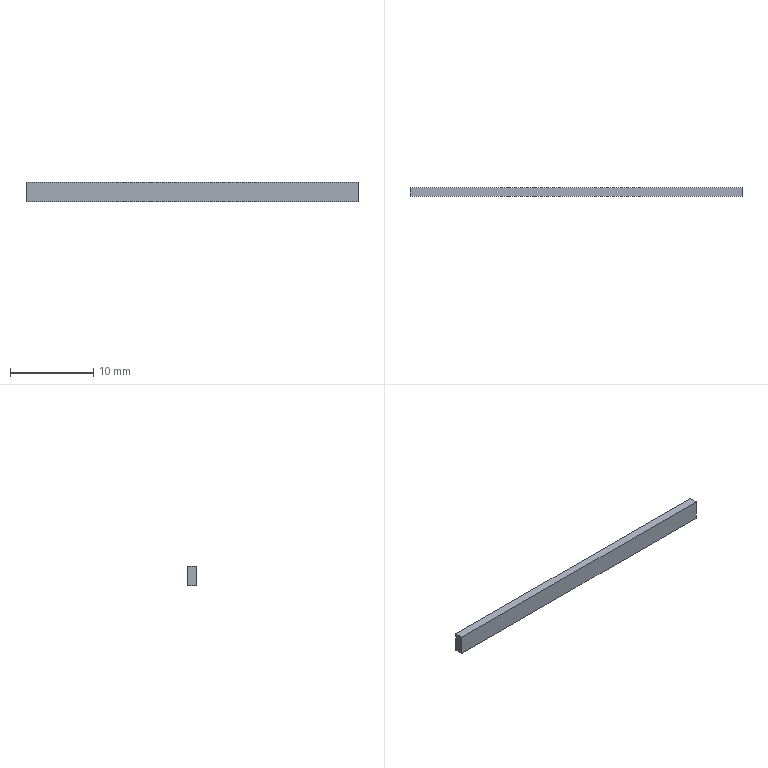Part | STEP file | TKR26H40-STAS | 1 solid | 6 faces | box 40 x 1 x 2.4 mm | volume 96 mm3 | plane 6
STEP:
#1=CARTESIAN_POINT('',(0.,0.,0.));
#2=DIRECTION('',(0.,0.,1.));
#3=DIRECTION('',(1.,0.,0.));
#4=AXIS2_PLACEMENT_3D('',#1,#2,#3);
#5=CARTESIAN_POINT('',(0.,40.,0.));
#6=VERTEX_POINT('',#5);
#7=CARTESIAN_POINT('',(0.,39.,0.));
#8=VERTEX_POINT('',#7);
#9=CARTESIAN_POINT('',(0.,39.5,0.));
#10=DIRECTION('',(0.,-1.,0.));
#11=VECTOR('',#10,1.);
#12=LINE('',#9,#11);
#13=CARTESIAN_POINT('',(20.,39.5,0.));
#14=DIRECTION('',(0.,0.,-1.));
#15=DIRECTION('',(0.,1.,0.));
#16=AXIS2_PLACEMENT_3D('',#13,#14,#15);
#17=PLANE('',#16);
#18=CARTESIAN_POINT('',(0.,-20.));
#19=DIRECTION('',(-1.,0.));
#20=VECTOR('',#19,1.);
#21=LINE('',#18,#20);
#22=(GEOMETRIC_REPRESENTATION_CONTEXT(2)PARAMETRIC_REPRESENTATION_CONTEXT()REPRESENTATION_CONTEXT('',''));
#23=DEFINITIONAL_REPRESENTATION('',(#21),#22);
#24=PCURVE('',#17,#23);
#25=CARTESIAN_POINT('',(0.,39.5,2.4));
#26=DIRECTION('',(-1.,0.,0.));
#27=DIRECTION('',(0.,0.,1.));
#28=AXIS2_PLACEMENT_3D('',#25,#26,#27);
#29=PLANE('',#28);
#30=CARTESIAN_POINT('',(-2.4,0.));
#31=DIRECTION('',(0.,-1.));
#32=VECTOR('',#31,1.);
#33=LINE('',#30,#32);
#34=(GEOMETRIC_REPRESENTATION_CONTEXT(2)PARAMETRIC_REPRESENTATION_CONTEXT()REPRESENTATION_CONTEXT('',''));
#35=DEFINITIONAL_REPRESENTATION('',(#33),#34);
#36=PCURVE('',#29,#35);
#37=SURFACE_CURVE('',#12,(#24,#36),.PCURVE_S1.);
#38=EDGE_CURVE('',#6,#8,#37,.T.);
#39=ORIENTED_EDGE('',*,*,#38,.F.);
#40=CARTESIAN_POINT('',(40.,40.,0.));
#41=VERTEX_POINT('',#40);
#42=CARTESIAN_POINT('',(20.,40.,0.));
#43=DIRECTION('',(-1.,0.,0.));
#44=VECTOR('',#43,1.);
#45=LINE('',#42,#44);
#46=CARTESIAN_POINT('',(0.5,0.));
#47=DIRECTION('',(0.,-1.));
#48=VECTOR('',#47,1.);
#49=LINE('',#46,#48);
#50=(GEOMETRIC_REPRESENTATION_CONTEXT(2)PARAMETRIC_REPRESENTATION_CONTEXT()REPRESENTATION_CONTEXT('',''));
#51=DEFINITIONAL_REPRESENTATION('',(#49),#50);
#52=PCURVE('',#17,#51);
#53=CARTESIAN_POINT('',(20.,40.,2.4));
#54=DIRECTION('',(0.,1.,0.));
#55=DIRECTION('',(0.,0.,1.));
#56=AXIS2_PLACEMENT_3D('',#53,#54,#55);
#57=PLANE('',#56);
#58=CARTESIAN_POINT('',(-2.4,0.));
#59=DIRECTION('',(0.,-1.));
#60=VECTOR('',#59,1.);
#61=LINE('',#58,#60);
#62=(GEOMETRIC_REPRESENTATION_CONTEXT(2)PARAMETRIC_REPRESENTATION_CONTEXT()REPRESENTATION_CONTEXT('',''));
#63=DEFINITIONAL_REPRESENTATION('',(#61),#62);
#64=PCURVE('',#57,#63);
#65=SURFACE_CURVE('',#45,(#52,#64),.PCURVE_S1.);
#66=EDGE_CURVE('',#41,#6,#65,.T.);
#67=ORIENTED_EDGE('',*,*,#66,.F.);
#68=CARTESIAN_POINT('',(40.,39.,0.));
#69=VERTEX_POINT('',#68);
#70=CARTESIAN_POINT('',(40.,39.5,0.));
#71=DIRECTION('',(0.,1.,0.));
#72=VECTOR('',#71,1.);
#73=LINE('',#70,#72);
#74=CARTESIAN_POINT('',(0.,20.));
#75=DIRECTION('',(1.,0.));
#76=VECTOR('',#75,1.);
#77=LINE('',#74,#76);
#78=(GEOMETRIC_REPRESENTATION_CONTEXT(2)PARAMETRIC_REPRESENTATION_CONTEXT()REPRESENTATION_CONTEXT('',''));
#79=DEFINITIONAL_REPRESENTATION('',(#77),#78);
#80=PCURVE('',#17,#79);
#81=CARTESIAN_POINT('',(40.,39.5,2.4));
#82=DIRECTION('',(1.,0.,0.));
#83=DIRECTION('',(0.,0.,-1.));
#84=AXIS2_PLACEMENT_3D('',#81,#82,#83);
#85=PLANE('',#84);
#86=CARTESIAN_POINT('',(2.4,0.));
#87=DIRECTION('',(0.,1.));
#88=VECTOR('',#87,1.);
#89=LINE('',#86,#88);
#90=(GEOMETRIC_REPRESENTATION_CONTEXT(2)PARAMETRIC_REPRESENTATION_CONTEXT()REPRESENTATION_CONTEXT('',''));
#91=DEFINITIONAL_REPRESENTATION('',(#89),#90);
#92=PCURVE('',#85,#91);
#93=SURFACE_CURVE('',#73,(#80,#92),.PCURVE_S1.);
#94=EDGE_CURVE('',#69,#41,#93,.T.);
#95=ORIENTED_EDGE('',*,*,#94,.F.);
#96=CARTESIAN_POINT('',(20.,39.,0.));
#97=DIRECTION('',(1.,0.,0.));
#98=VECTOR('',#97,1.);
#99=LINE('',#96,#98);
#100=CARTESIAN_POINT('',(-0.5,0.));
#101=DIRECTION('',(0.,1.));
#102=VECTOR('',#101,1.);
#103=LINE('',#100,#102);
#104=(GEOMETRIC_REPRESENTATION_CONTEXT(2)PARAMETRIC_REPRESENTATION_CONTEXT()REPRESENTATION_CONTEXT('',''));
#105=DEFINITIONAL_REPRESENTATION('',(#103),#104);
#106=PCURVE('',#17,#105);
#107=CARTESIAN_POINT('',(20.,39.,2.4));
#108=DIRECTION('',(0.,-1.,0.));
#109=DIRECTION('',(0.,0.,-1.));
#110=AXIS2_PLACEMENT_3D('',#107,#108,#109);
#111=PLANE('',#110);
#112=CARTESIAN_POINT('',(2.4,0.));
#113=DIRECTION('',(0.,1.));
#114=VECTOR('',#113,1.);
#115=LINE('',#112,#114);
#116=(GEOMETRIC_REPRESENTATION_CONTEXT(2)PARAMETRIC_REPRESENTATION_CONTEXT()REPRESENTATION_CONTEXT('',''));
#117=DEFINITIONAL_REPRESENTATION('',(#115),#116);
#118=PCURVE('',#111,#117);
#119=SURFACE_CURVE('',#99,(#106,#118),.PCURVE_S1.);
#120=EDGE_CURVE('',#8,#69,#119,.T.);
#121=ORIENTED_EDGE('',*,*,#120,.F.);
#122=EDGE_LOOP('',(#39,#67,#95,#121));
#123=FACE_BOUND('',#122,.T.);
#124=ADVANCED_FACE('',(#123),#17,.T.);
#125=CARTESIAN_POINT('',(0.,40.,2.4));
#126=VERTEX_POINT('',#125);
#127=CARTESIAN_POINT('',(0.,40.,2.4));
#128=DIRECTION('',(0.,0.,-1.));
#129=VECTOR('',#128,1.);
#130=LINE('',#127,#129);
#131=CARTESIAN_POINT('',(0.,0.5));
#132=DIRECTION('',(-1.,0.));
#133=VECTOR('',#132,1.);
#134=LINE('',#131,#133);
#135=(GEOMETRIC_REPRESENTATION_CONTEXT(2)PARAMETRIC_REPRESENTATION_CONTEXT()REPRESENTATION_CONTEXT('',''));
#136=DEFINITIONAL_REPRESENTATION('',(#134),#135);
#137=PCURVE('',#29,#136);
#138=CARTESIAN_POINT('',(0.,-20.));
#139=DIRECTION('',(-1.,0.));
#140=VECTOR('',#139,1.);
#141=LINE('',#138,#140);
#142=(GEOMETRIC_REPRESENTATION_CONTEXT(2)PARAMETRIC_REPRESENTATION_CONTEXT()REPRESENTATION_CONTEXT('',''));
#143=DEFINITIONAL_REPRESENTATION('',(#141),#142);
#144=PCURVE('',#57,#143);
#145=SURFACE_CURVE('',#130,(#137,#144),.PCURVE_S1.);
#146=EDGE_CURVE('',#126,#6,#145,.T.);
#147=ORIENTED_EDGE('',*,*,#146,.T.);
#148=ORIENTED_EDGE('',*,*,#38,.T.);
#149=CARTESIAN_POINT('',(0.,39.,2.4));
#150=VERTEX_POINT('',#149);
#151=CARTESIAN_POINT('',(0.,39.,2.4));
#152=DIRECTION('',(0.,0.,-1.));
#153=VECTOR('',#152,1.);
#154=LINE('',#151,#153);
#155=CARTESIAN_POINT('',(0.,-0.5));
#156=DIRECTION('',(-1.,0.));
#157=VECTOR('',#156,1.);
#158=LINE('',#155,#157);
#159=(GEOMETRIC_REPRESENTATION_CONTEXT(2)PARAMETRIC_REPRESENTATION_CONTEXT()REPRESENTATION_CONTEXT('',''));
#160=DEFINITIONAL_REPRESENTATION('',(#158),#159);
#161=PCURVE('',#29,#160);
#162=CARTESIAN_POINT('',(0.,-20.));
#163=DIRECTION('',(1.,0.));
#164=VECTOR('',#163,1.);
#165=LINE('',#162,#164);
#166=(GEOMETRIC_REPRESENTATION_CONTEXT(2)PARAMETRIC_REPRESENTATION_CONTEXT()REPRESENTATION_CONTEXT('',''));
#167=DEFINITIONAL_REPRESENTATION('',(#165),#166);
#168=PCURVE('',#111,#167);
#169=SURFACE_CURVE('',#154,(#161,#168),.PCURVE_S1.);
#170=EDGE_CURVE('',#150,#8,#169,.T.);
#171=ORIENTED_EDGE('',*,*,#170,.F.);
#172=CARTESIAN_POINT('',(0.,39.5,2.4));
#173=DIRECTION('',(0.,1.,0.));
#174=VECTOR('',#173,1.);
#175=LINE('',#172,#174);
#176=CARTESIAN_POINT('',(0.,0.));
#177=DIRECTION('',(0.,1.));
#178=VECTOR('',#177,1.);
#179=LINE('',#176,#178);
#180=(GEOMETRIC_REPRESENTATION_CONTEXT(2)PARAMETRIC_REPRESENTATION_CONTEXT()REPRESENTATION_CONTEXT('',''));
#181=DEFINITIONAL_REPRESENTATION('',(#179),#180);
#182=PCURVE('',#29,#181);
#183=CARTESIAN_POINT('',(20.,39.5,2.4));
#184=DIRECTION('',(0.,0.,1.));
#185=DIRECTION('',(0.,-1.,0.));
#186=AXIS2_PLACEMENT_3D('',#183,#184,#185);
#187=PLANE('',#186);
#188=CARTESIAN_POINT('',(0.,-20.));
#189=DIRECTION('',(-1.,0.));
#190=VECTOR('',#189,1.);
#191=LINE('',#188,#190);
#192=(GEOMETRIC_REPRESENTATION_CONTEXT(2)PARAMETRIC_REPRESENTATION_CONTEXT()REPRESENTATION_CONTEXT('',''));
#193=DEFINITIONAL_REPRESENTATION('',(#191),#192);
#194=PCURVE('',#187,#193);
#195=SURFACE_CURVE('',#175,(#182,#194),.PCURVE_S1.);
#196=EDGE_CURVE('',#150,#126,#195,.T.);
#197=ORIENTED_EDGE('',*,*,#196,.T.);
#198=EDGE_LOOP('',(#147,#148,#171,#197));
#199=FACE_BOUND('',#198,.T.);
#200=ADVANCED_FACE('',(#199),#29,.T.);
#201=ORIENTED_EDGE('',*,*,#170,.T.);
#202=ORIENTED_EDGE('',*,*,#120,.T.);
#203=CARTESIAN_POINT('',(40.,39.,2.4));
#204=VERTEX_POINT('',#203);
#205=CARTESIAN_POINT('',(40.,39.,2.4));
#206=DIRECTION('',(0.,0.,-1.));
#207=VECTOR('',#206,1.);
#208=LINE('',#205,#207);
#209=CARTESIAN_POINT('',(0.,20.));
#210=DIRECTION('',(1.,0.));
#211=VECTOR('',#210,1.);
#212=LINE('',#209,#211);
#213=(GEOMETRIC_REPRESENTATION_CONTEXT(2)PARAMETRIC_REPRESENTATION_CONTEXT()REPRESENTATION_CONTEXT('',''));
#214=DEFINITIONAL_REPRESENTATION('',(#212),#213);
#215=PCURVE('',#111,#214);
#216=CARTESIAN_POINT('',(0.,-0.5));
#217=DIRECTION('',(1.,0.));
#218=VECTOR('',#217,1.);
#219=LINE('',#216,#218);
#220=(GEOMETRIC_REPRESENTATION_CONTEXT(2)PARAMETRIC_REPRESENTATION_CONTEXT()REPRESENTATION_CONTEXT('',''));
#221=DEFINITIONAL_REPRESENTATION('',(#219),#220);
#222=PCURVE('',#85,#221);
#223=SURFACE_CURVE('',#208,(#215,#222),.PCURVE_S1.);
#224=EDGE_CURVE('',#204,#69,#223,.T.);
#225=ORIENTED_EDGE('',*,*,#224,.F.);
#226=CARTESIAN_POINT('',(20.,39.,2.4));
#227=DIRECTION('',(-1.,0.,0.));
#228=VECTOR('',#227,1.);
#229=LINE('',#226,#228);
#230=CARTESIAN_POINT('',(0.,0.));
#231=DIRECTION('',(0.,-1.));
#232=VECTOR('',#231,1.);
#233=LINE('',#230,#232);
#234=(GEOMETRIC_REPRESENTATION_CONTEXT(2)PARAMETRIC_REPRESENTATION_CONTEXT()REPRESENTATION_CONTEXT('',''));
#235=DEFINITIONAL_REPRESENTATION('',(#233),#234);
#236=PCURVE('',#111,#235);
#237=CARTESIAN_POINT('',(0.5,0.));
#238=DIRECTION('',(0.,-1.));
#239=VECTOR('',#238,1.);
#240=LINE('',#237,#239);
#241=(GEOMETRIC_REPRESENTATION_CONTEXT(2)PARAMETRIC_REPRESENTATION_CONTEXT()REPRESENTATION_CONTEXT('',''));
#242=DEFINITIONAL_REPRESENTATION('',(#240),#241);
#243=PCURVE('',#187,#242);
#244=SURFACE_CURVE('',#229,(#236,#243),.PCURVE_S1.);
#245=EDGE_CURVE('',#204,#150,#244,.T.);
#246=ORIENTED_EDGE('',*,*,#245,.T.);
#247=EDGE_LOOP('',(#201,#202,#225,#246));
#248=FACE_BOUND('',#247,.T.);
#249=ADVANCED_FACE('',(#248),#111,.T.);
#250=ORIENTED_EDGE('',*,*,#224,.T.);
#251=ORIENTED_EDGE('',*,*,#94,.T.);
#252=CARTESIAN_POINT('',(40.,40.,2.4));
#253=VERTEX_POINT('',#252);
#254=CARTESIAN_POINT('',(40.,40.,2.4));
#255=DIRECTION('',(0.,0.,-1.));
#256=VECTOR('',#255,1.);
#257=LINE('',#254,#256);
#258=CARTESIAN_POINT('',(0.,0.5));
#259=DIRECTION('',(1.,0.));
#260=VECTOR('',#259,1.);
#261=LINE('',#258,#260);
#262=(GEOMETRIC_REPRESENTATION_CONTEXT(2)PARAMETRIC_REPRESENTATION_CONTEXT()REPRESENTATION_CONTEXT('',''));
#263=DEFINITIONAL_REPRESENTATION('',(#261),#262);
#264=PCURVE('',#85,#263);
#265=CARTESIAN_POINT('',(0.,20.));
#266=DIRECTION('',(-1.,0.));
#267=VECTOR('',#266,1.);
#268=LINE('',#265,#267);
#269=(GEOMETRIC_REPRESENTATION_CONTEXT(2)PARAMETRIC_REPRESENTATION_CONTEXT()REPRESENTATION_CONTEXT('',''));
#270=DEFINITIONAL_REPRESENTATION('',(#268),#269);
#271=PCURVE('',#57,#270);
#272=SURFACE_CURVE('',#257,(#264,#271),.PCURVE_S1.);
#273=EDGE_CURVE('',#253,#41,#272,.T.);
#274=ORIENTED_EDGE('',*,*,#273,.F.);
#275=CARTESIAN_POINT('',(40.,39.5,2.4));
#276=DIRECTION('',(0.,-1.,0.));
#277=VECTOR('',#276,1.);
#278=LINE('',#275,#277);
#279=CARTESIAN_POINT('',(0.,0.));
#280=DIRECTION('',(0.,-1.));
#281=VECTOR('',#280,1.);
#282=LINE('',#279,#281);
#283=(GEOMETRIC_REPRESENTATION_CONTEXT(2)PARAMETRIC_REPRESENTATION_CONTEXT()REPRESENTATION_CONTEXT('',''));
#284=DEFINITIONAL_REPRESENTATION('',(#282),#283);
#285=PCURVE('',#85,#284);
#286=CARTESIAN_POINT('',(0.,20.));
#287=DIRECTION('',(1.,0.));
#288=VECTOR('',#287,1.);
#289=LINE('',#286,#288);
#290=(GEOMETRIC_REPRESENTATION_CONTEXT(2)PARAMETRIC_REPRESENTATION_CONTEXT()REPRESENTATION_CONTEXT('',''));
#291=DEFINITIONAL_REPRESENTATION('',(#289),#290);
#292=PCURVE('',#187,#291);
#293=SURFACE_CURVE('',#278,(#285,#292),.PCURVE_S1.);
#294=EDGE_CURVE('',#253,#204,#293,.T.);
#295=ORIENTED_EDGE('',*,*,#294,.T.);
#296=EDGE_LOOP('',(#250,#251,#274,#295));
#297=FACE_BOUND('',#296,.T.);
#298=ADVANCED_FACE('',(#297),#85,.T.);
#299=CARTESIAN_POINT('',(20.,40.,2.4));
#300=DIRECTION('',(1.,0.,0.));
#301=VECTOR('',#300,1.);
#302=LINE('',#299,#301);
#303=CARTESIAN_POINT('',(-0.5,0.));
#304=DIRECTION('',(0.,1.));
#305=VECTOR('',#304,1.);
#306=LINE('',#303,#305);
#307=(GEOMETRIC_REPRESENTATION_CONTEXT(2)PARAMETRIC_REPRESENTATION_CONTEXT()REPRESENTATION_CONTEXT('',''));
#308=DEFINITIONAL_REPRESENTATION('',(#306),#307);
#309=PCURVE('',#187,#308);
#310=CARTESIAN_POINT('',(0.,0.));
#311=DIRECTION('',(0.,1.));
#312=VECTOR('',#311,1.);
#313=LINE('',#310,#312);
#314=(GEOMETRIC_REPRESENTATION_CONTEXT(2)PARAMETRIC_REPRESENTATION_CONTEXT()REPRESENTATION_CONTEXT('',''));
#315=DEFINITIONAL_REPRESENTATION('',(#313),#314);
#316=PCURVE('',#57,#315);
#317=SURFACE_CURVE('',#302,(#309,#316),.PCURVE_S1.);
#318=EDGE_CURVE('',#126,#253,#317,.T.);
#319=ORIENTED_EDGE('',*,*,#318,.F.);
#320=ORIENTED_EDGE('',*,*,#196,.F.);
#321=ORIENTED_EDGE('',*,*,#245,.F.);
#322=ORIENTED_EDGE('',*,*,#294,.F.);
#323=EDGE_LOOP('',(#319,#320,#321,#322));
#324=FACE_BOUND('',#323,.T.);
#325=ADVANCED_FACE('',(#324),#187,.T.);
#326=ORIENTED_EDGE('',*,*,#318,.T.);
#327=ORIENTED_EDGE('',*,*,#273,.T.);
#328=ORIENTED_EDGE('',*,*,#66,.T.);
#329=ORIENTED_EDGE('',*,*,#146,.F.);
#330=EDGE_LOOP('',(#326,#327,#328,#329));
#331=FACE_BOUND('',#330,.T.);
#332=ADVANCED_FACE('',(#331),#57,.T.);
#333=CLOSED_SHELL('',(#124,#200,#249,#298,#325,#332));
#334=MANIFOLD_SOLID_BREP('',#333);
#335=(LENGTH_UNIT()NAMED_UNIT(*)SI_UNIT(.MILLI.,.METRE.));
#336=UNCERTAINTY_MEASURE_WITH_UNIT(LENGTH_MEASURE(0.0000001),#335,'','');
#337=(NAMED_UNIT(*)PLANE_ANGLE_UNIT()SI_UNIT($,.RADIAN.));
#338=(NAMED_UNIT(*)SI_UNIT($,.STERADIAN.)SOLID_ANGLE_UNIT());
#339=(GEOMETRIC_REPRESENTATION_CONTEXT(3)GLOBAL_UNCERTAINTY_ASSIGNED_CONTEXT((#336))GLOBAL_UNIT_ASSIGNED_CONTEXT((#335,#337,#338))REPRESENTATION_CONTEXT('',''));
#340=ADVANCED_BREP_SHAPE_REPRESENTATION('',(#4,#334),#339);